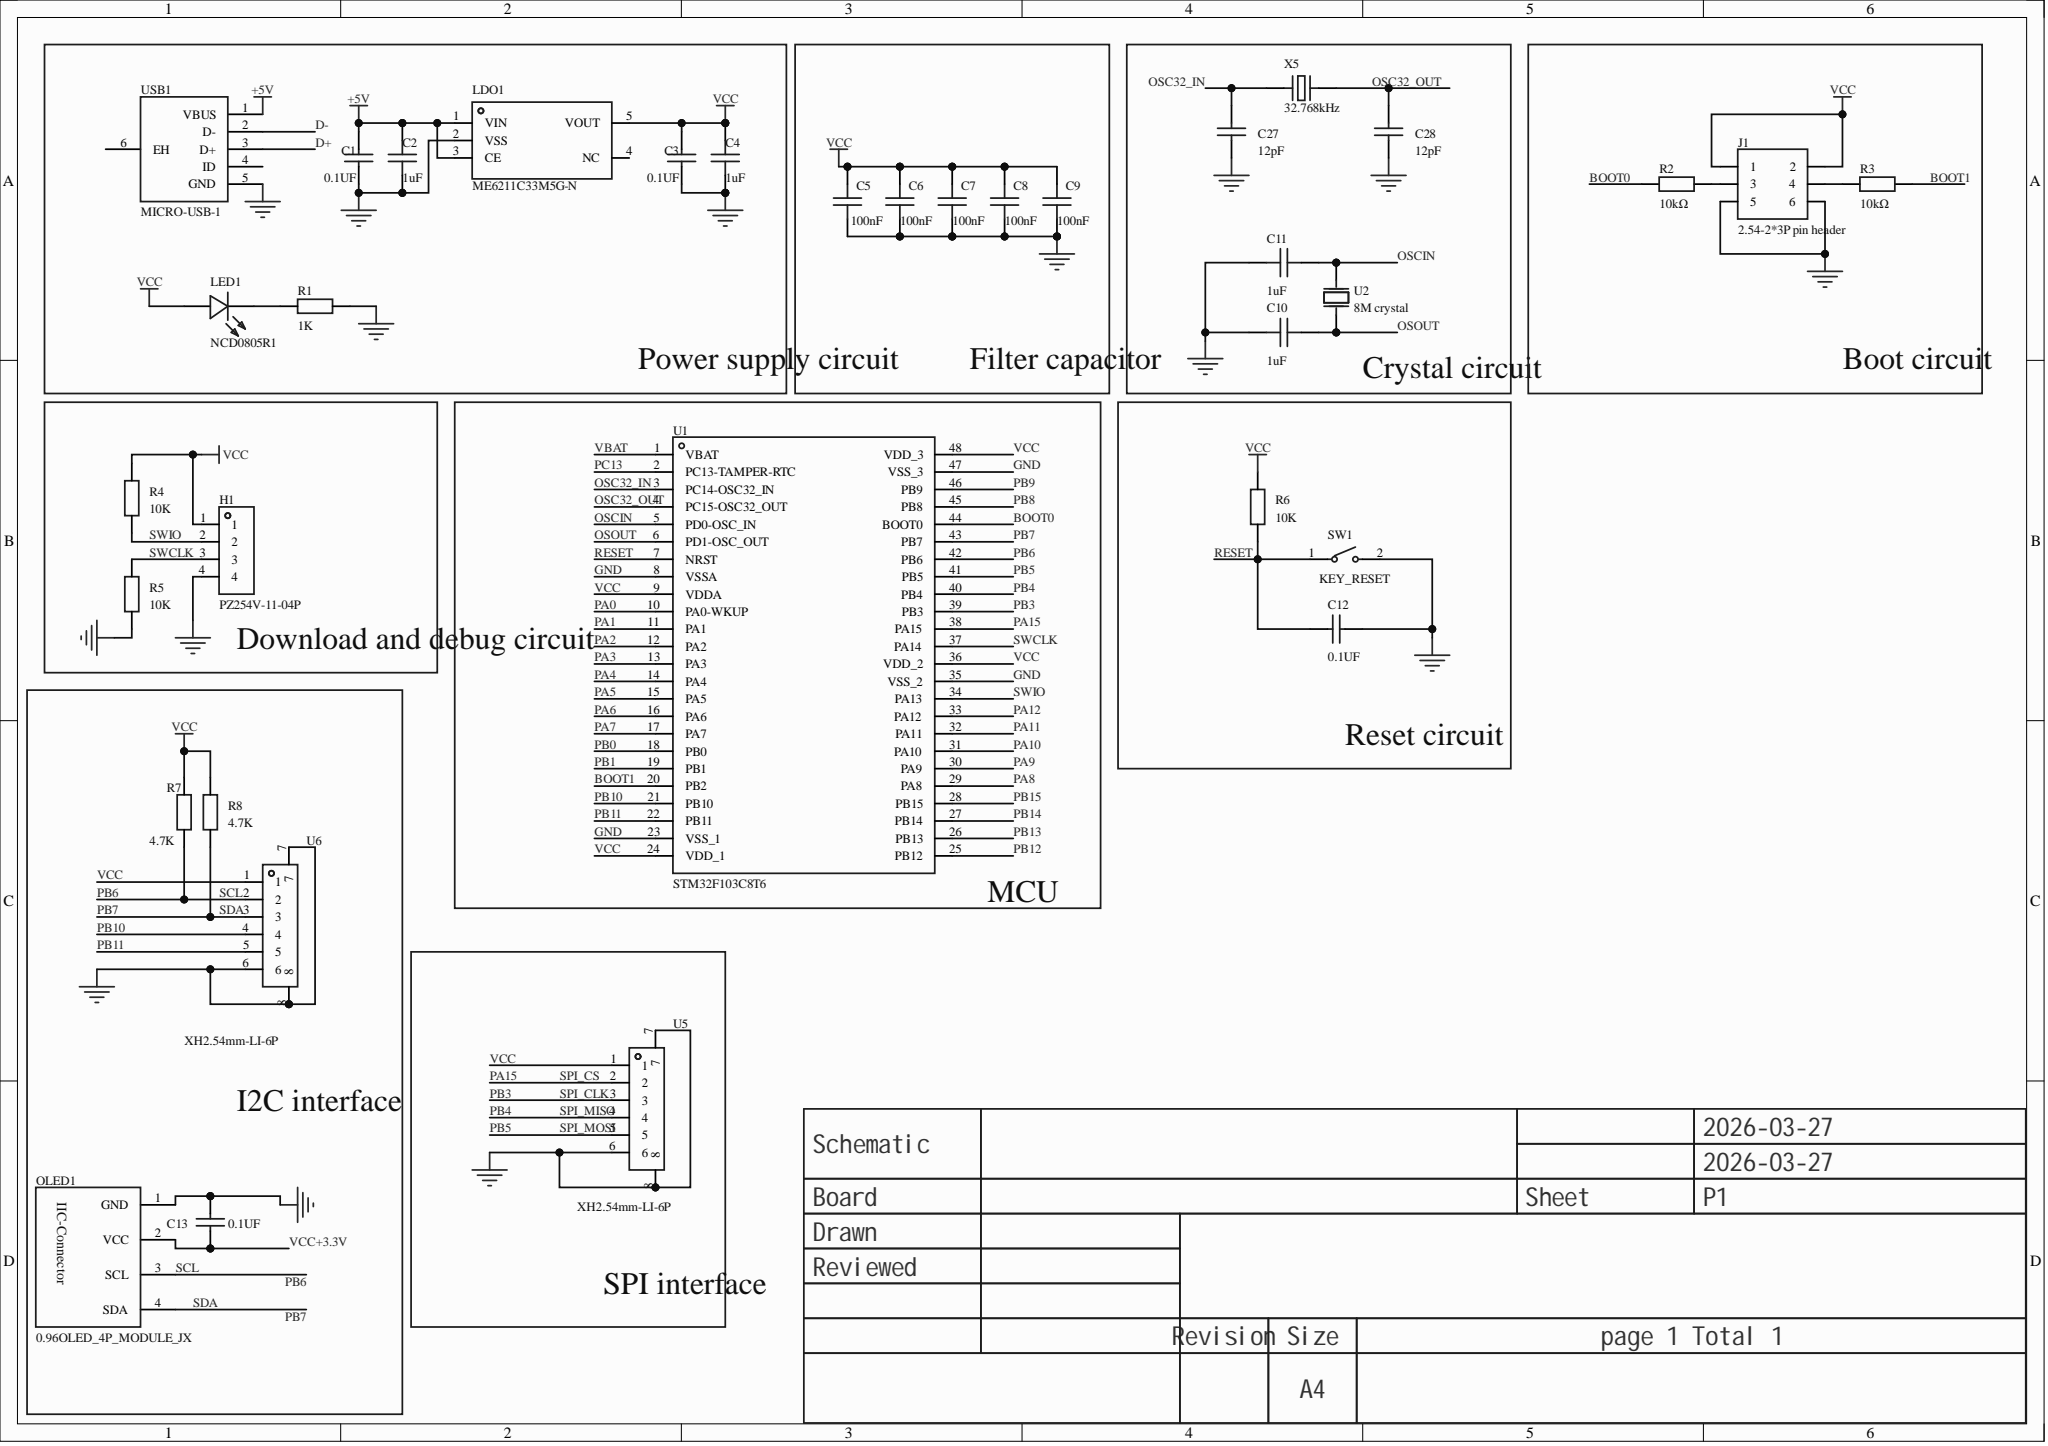Circuit board | Altium Designer | 35 parts | 24 nets
Bill of materials:
Comment,Description,Designator,Footprint,LibRef,Quantity
"0.1UF","","C1, C3, C12, C13","C0603","CAPCER0.1UF16VX5R0603,CAPCER0.1UF25VX5R0603,CAPCER0.1UF16VX7R0603","4"
"1uF","Capacitance:1uF;Tolerance:±10%;Rated voltage:50V;Temperature coefficient:X5R;","C2, C4, C10, C11","C0603","CL10A105KB8NNNC","4"
"100nF","Capacitance:100nF;Tolerance:±10%;Rated voltage:16V;Temperature coefficient:X7R;","C5, C6, C7, C8, C9","C0603","CC0603KPX7R7BB104","5"
"12pF","Capacitance:12pF;Tolerance:±5%;Rated voltage:50V;Material (temperature coefficient):C0G;","C27, C28","R0402","0402CG120J500NT","2"
"PZ254V-11-04P","Pin structure:1x4P;Pitch:2.54mm;Row spacing:-;Round/square pin:Square;Mounting:Through-hole;Rows:Single row;Total pin count:4P;Rated current:3A;Rated voltage:250V;Mating pin length:6mm;Plastic height:2.5mm;Terminal pin length:3mm;Contact material:-;Operating temperature:-40℃~+105℃;Color:Black;","H1","HDR-TH_4P-P2.54-V-M","PZ254V-11-04P","1"
"2.54-2*3P pin header","Pin structure:-;Pitch:2.54mm;Row spacing:2.54mm;Round/square pin:-;Mounting:Through-hole;Rows:Dual row;Total pin count:6P;Rated current:-;Rated voltage:-;Mating pin length:-;Plastic height:-;Contact material:-;Contact plating:-;Color:Black;","J1","HDR-TH_6P-P2.54-V-M-R2-C3-S2.54-1","2.54-2*3P针","1"
"ME6211C33M5G-N","Output type:Fixed;Operating voltage:6V;Output voltage:3.3V;Output current:500mA;PSRR:70dB@(1kHz);Output polarity:Positive;","LDO1","SOT-23-5_L3.0-W1.7-P0.95-LS2.8-BL","ME6211C33M5G-N","1"
"NCD0805R1","Lamp head type:-;Emission color:Red;Forward voltage drop (Vf):1.6V~2.6V;Power:65mW;Forward current:25mA;Wavelength:615nm~630nm;Diode configuration:Discrete diode;Lens color:-;Color temperature:-;Luminous intensity:195mcd;Viewing angle:130°;Packaging:-;Operating temperature:-30℃~+85℃;","LED1","LED0805-RD","NCD0805R1","1"
"0.96OLED_4P_MODULE_JX","","OLED1","0.96OLED_4P","0.96OLED_4P_MODULE_JX","1"
"1K","","R1","R0603","Res_0603","1"
"10kΩ","Resistor type:Thick-film resistor;Resistance:10kΩ;Tolerance:±1%;Power:100mW;Operating voltage:75V;Temperature coefficient:±100ppm/?;","R2, R3","R0603","0603WAF1002T5E","2"
"10K","","R4, R5, R6","R0603","Res_0603","3"
"4.7K","","R7, R8","R0603","Res_0603","2"
"KEY_RESET","","SW1","SW-SMD_L6.0-W3.3-LS8.0","SW_PB2_A1","1"
"STM32F103C8T6","CPU core:ARM-M3;Max CPU frequency:72MHz;Application field:-;","U1","LQFP-48_L7.0-W7.0-P0.50-LS9.0-BL","STM32F103C8T6","1"
"8M crystal","","U2","HC-49S_L11.5-W4.7-P4.88","8M晶振_C9900011272","1"
"XH2.54mm-LI-6P","","U5, U6","CONN-SMD_6P-P2.50-H","XH2.54mm-LI-6P","2"
"MICRO-USB-1","","USB1","MICRO-USB-SMD_C9900008946","MICRO-USB-1","1"
"32.768kHz","Crystal type:SMD crystal;Frequency:32.768kHz;Frequency deviation at room temp:±20ppm;External load capacitance:12.5pF;Frequency stability (full temp):-;","X5","OSC-SMD_L3.2-W1.5","X321532768KGD2SI","1"
Netlist (Protel format):
[
C1
C0603
0.1UF



]
[
C2
C0603
1uF



]
[
C3
C0603
0.1UF



]
[
C4
C0603
1uF



]
[
C5
C0603
100nF



]
[
C6
C0603
100nF



]
[
C7
C0603
100nF



]
[
C8
C0603
100nF



]
[
C9
C0603
100nF



]
[
C10
C0603
1uF



]
[
C11
C0603
1uF



]
[
C12
C0603
0.1UF



]
[
C13
C0603
0.1UF



]
[
C27
R0402
12pF



]
[
C28
R0402
12pF



]
[
H1
HDR-TH_4P-P2.54-V-M
PZ254V-11-04P



]
[
J1
HDR-TH_6P-P2.54-V-M-R2-C3-S2.54-1
2.54-2*3P pin header



]
[
LDO1
SOT-23-5_L3.0-W1.7-P0.95-LS2.8-BL
ME6211C33M5G-N



]
[
LED1
LED0805-RD
NCD0805R1



]
[
OLED1
0.96OLED_4P
0.96OLED_4P_MODULE_JX



]
[
R1
R0603
1K



]
[
R2
R0603
10kΩ



]
[
R3
R0603
10kΩ



]
[
R4
R0603
10K



]
[
R5
R0603
10K



]
[
R6
R0603
10K



]
[
R7
R0603
4.7K



]
[
R8
R0603
4.7K



]
[
SW1
SW-SMD_L6.0-W3.3-LS8.0
KEY_RESET



]
[
U1
LQFP-48_L7.0-W7.0-P0.50-LS9.0-BL
STM32F103C8T6



]
[
U2
HC-49S_L11.5-W4.7-P4.88
8M crystal



]
[
U5
CONN-SMD_6P-P2.50-H
XH2.54mm-LI-6P



]
[
U6
CONN-SMD_6P-P2.50-H
XH2.54mm-LI-6P



]
[
USB1
MICRO-USB-SMD_C9900008946
MICRO-USB-1



]
[
X5
OSC-SMD_L3.2-W1.5
32.768kHz



]
(
VCC+3.3V
C13-1
OLED1-2
)
(
VCC
C3-2
C4-2
C5-2
C6-2
C7-2
C8-2
C9-2
H1-1
J1-1
J1-2
LDO1-5
LED1-2
R4-2
R6-2
R7-2
R8-2
U1-9
U1-24
U1-36
U1-48
U5-1
U6-1
)
(
SWIO
H1-2
R4-1
U1-34
)
(
SWCLK
H1-3
R5-2
U1-37
)
(
RESET
C12-2
R6-1
SW1-1
U1-7
)
(
PB11
U1-22
U6-5
)
(
PB10
U1-21
U6-4
)
(
PB7
OLED1-4
R8-1
U1-43
U6-3
)
(
PB6
OLED1-3
R7-1
U1-42
U6-2
)
(
PB5
U1-41
U5-5
)
(
PB4
U1-40
U5-4
)
(
PB3
U1-39
U5-3
)
(
PA15
U1-38
U5-2
)
(
OSOUT
C10-1
U1-6
U2-2
)
(
OSCIN
C11-1
U1-5
U2-1
)
(
OSC32_OUT
C28-2
U1-4
X5-2
)
(
OSC32_IN
C27-2
U1-3
X5-1
)
(
NetLED1_1
LED1-1
R1-1
)
(
NetJ1_4
J1-4
R3-1
)
(
NetJ1_3
J1-3
R2-2
)
(
GND
C1-1
C2-1
C3-1
C4-1
C5-1
C6-1
C7-1
C8-1
C9-1
C10-2
C11-2
C12-1
C13-2
C27-1
C28-1
H1-4
J1-5
J1-6
LDO1-2
OLED1-1
R1-2
R5-1
SW1-2
U1-8
U1-23
U1-35
U1-47
U5-6
U5-7
U5-8
U6-6
U6-7
U6-8
USB1-5
)
(
BOOT1
R3-2
U1-20
)
(
BOOT0
R2-1
U1-44
)
(
+5V
C1-2
C2-2
LDO1-1
LDO1-3
USB1-1
)